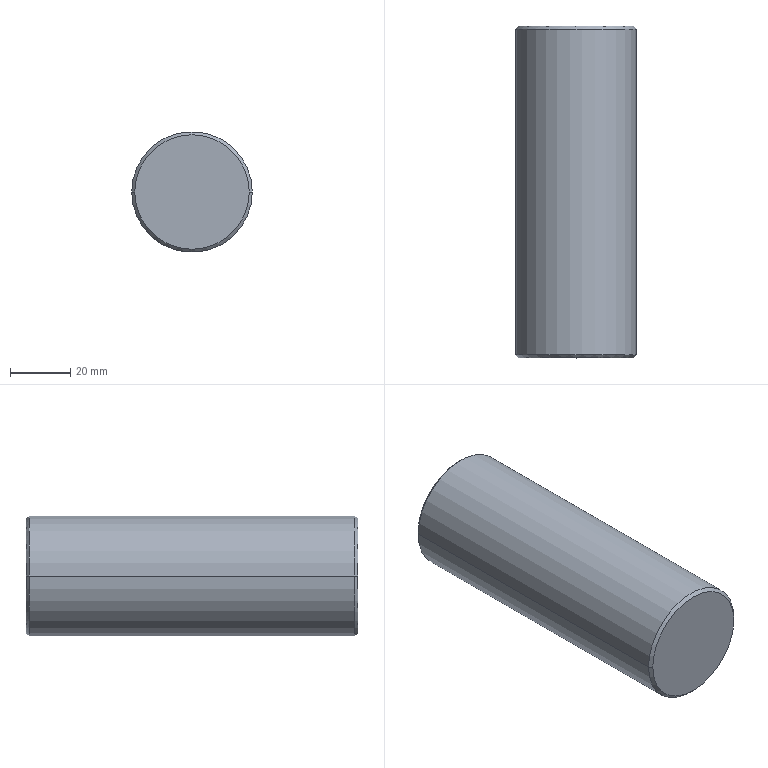Part | SolidWorks | 1 solid | 8 faces | box 40 x 110 x 40 mm | volume 138107 mm3 | cone 4 | cylinder 2 | plane 2 | commonest cylinder face diameters 40 x2
STEP:
#1=CARTESIAN_POINT('',(-19.,0.,0.));
#2=VERTEX_POINT('',#1);
#3=CARTESIAN_POINT('',(19.,0.,0.));
#4=VERTEX_POINT('',#3);
#5=CARTESIAN_POINT('',(0.,0.,0.));
#6=DIRECTION('',(0.,1.,0.));
#7=DIRECTION('',(-1.,0.,0.));
#8=AXIS2_PLACEMENT_3D('',#5,#6,#7);
#9=CIRCLE('',#8,19.);
#10=EDGE_CURVE('',#2,#4,#9,.T.);
#11=ORIENTED_EDGE('',*,*,#10,.F.);
#12=CARTESIAN_POINT('',(-20.,-1.,0.));
#13=VERTEX_POINT('',#12);
#14=CARTESIAN_POINT('',(-20.,-1.,0.));
#15=DIRECTION('',(-0.7071,-0.7071,0.));
#16=VECTOR('',#15,1000.);
#17=LINE('',#14,#16);
#18=EDGE_CURVE('',#2,#13,#17,.T.);
#19=ORIENTED_EDGE('',*,*,#18,.T.);
#20=CARTESIAN_POINT('',(20.,-1.,0.));
#21=VERTEX_POINT('',#20);
#22=CARTESIAN_POINT('',(0.,-1.,0.));
#23=DIRECTION('',(0.,1.,0.));
#24=DIRECTION('',(-1.,0.,0.));
#25=AXIS2_PLACEMENT_3D('',#22,#23,#24);
#26=CIRCLE('',#25,20.);
#27=EDGE_CURVE('',#13,#21,#26,.T.);
#28=ORIENTED_EDGE('',*,*,#27,.T.);
#29=CARTESIAN_POINT('',(20.,-1.,0.));
#30=DIRECTION('',(0.7071,-0.7071,0.));
#31=VECTOR('',#30,1000.);
#32=LINE('',#29,#31);
#33=EDGE_CURVE('',#4,#21,#32,.T.);
#34=ORIENTED_EDGE('',*,*,#33,.F.);
#35=EDGE_LOOP('',(#11,#19,#28,#34));
#36=FACE_OUTER_BOUND('',#35,.T.);
#37=CARTESIAN_POINT('',(0.,-1.,0.));
#38=DIRECTION('',(0.,-1.,0.));
#39=DIRECTION('',(1.,0.,0.));
#40=AXIS2_PLACEMENT_3D('',#37,#38,#39);
#41=CONICAL_SURFACE('',#40,20.,0.7854);
#42=ADVANCED_FACE('',(#36),#41,.T.);
#43=CARTESIAN_POINT('',(-20.,-109.,0.));
#44=VERTEX_POINT('',#43);
#45=CARTESIAN_POINT('',(20.,-109.,0.));
#46=VERTEX_POINT('',#45);
#47=CARTESIAN_POINT('',(0.,-109.,0.));
#48=DIRECTION('',(0.,1.,0.));
#49=DIRECTION('',(-1.,0.,0.));
#50=AXIS2_PLACEMENT_3D('',#47,#48,#49);
#51=CIRCLE('',#50,20.);
#52=EDGE_CURVE('',#44,#46,#51,.T.);
#53=ORIENTED_EDGE('',*,*,#52,.T.);
#54=CARTESIAN_POINT('',(20.,0.,0.));
#55=DIRECTION('',(0.,1.,0.));
#56=VECTOR('',#55,1000.);
#57=LINE('',#54,#56);
#58=EDGE_CURVE('',#46,#21,#57,.T.);
#59=ORIENTED_EDGE('',*,*,#58,.T.);
#60=ORIENTED_EDGE('',*,*,#27,.F.);
#61=CARTESIAN_POINT('',(-20.,0.,0.));
#62=DIRECTION('',(0.,1.,0.));
#63=VECTOR('',#62,1000.);
#64=LINE('',#61,#63);
#65=EDGE_CURVE('',#44,#13,#64,.T.);
#66=ORIENTED_EDGE('',*,*,#65,.F.);
#67=EDGE_LOOP('',(#53,#59,#60,#66));
#68=FACE_OUTER_BOUND('',#67,.T.);
#69=CARTESIAN_POINT('',(0.,0.,0.));
#70=DIRECTION('',(0.,1.,0.));
#71=DIRECTION('',(-1.,0.,0.));
#72=AXIS2_PLACEMENT_3D('',#69,#70,#71);
#73=CYLINDRICAL_SURFACE('',#72,20.);
#74=ADVANCED_FACE('',(#68),#73,.T.);
#75=CARTESIAN_POINT('',(-19.,-110.,0.));
#76=VERTEX_POINT('',#75);
#77=CARTESIAN_POINT('',(19.,-110.,0.));
#78=VERTEX_POINT('',#77);
#79=CARTESIAN_POINT('',(0.,-110.,0.));
#80=DIRECTION('',(0.,1.,0.));
#81=DIRECTION('',(-1.,0.,0.));
#82=AXIS2_PLACEMENT_3D('',#79,#80,#81);
#83=CIRCLE('',#82,19.);
#84=EDGE_CURVE('',#76,#78,#83,.T.);
#85=ORIENTED_EDGE('',*,*,#84,.T.);
#86=CARTESIAN_POINT('',(19.,-110.,0.));
#87=DIRECTION('',(0.7071,0.7071,0.));
#88=VECTOR('',#87,1000.);
#89=LINE('',#86,#88);
#90=EDGE_CURVE('',#78,#46,#89,.T.);
#91=ORIENTED_EDGE('',*,*,#90,.T.);
#92=ORIENTED_EDGE('',*,*,#52,.F.);
#93=CARTESIAN_POINT('',(-19.,-110.,0.));
#94=DIRECTION('',(-0.7071,0.7071,0.));
#95=VECTOR('',#94,1000.);
#96=LINE('',#93,#95);
#97=EDGE_CURVE('',#76,#44,#96,.T.);
#98=ORIENTED_EDGE('',*,*,#97,.F.);
#99=EDGE_LOOP('',(#85,#91,#92,#98));
#100=FACE_OUTER_BOUND('',#99,.T.);
#101=CARTESIAN_POINT('',(0.,-110.,0.));
#102=DIRECTION('',(0.,1.,0.));
#103=DIRECTION('',(-1.,0.,0.));
#104=AXIS2_PLACEMENT_3D('',#101,#102,#103);
#105=CONICAL_SURFACE('',#104,19.,0.7854);
#106=ADVANCED_FACE('',(#100),#105,.T.);
#107=ORIENTED_EDGE('',*,*,#84,.F.);
#108=CARTESIAN_POINT('',(0.,-110.,0.));
#109=DIRECTION('',(0.,1.,0.));
#110=DIRECTION('',(-1.,0.,0.));
#111=AXIS2_PLACEMENT_3D('',#108,#109,#110);
#112=CIRCLE('',#111,19.);
#113=EDGE_CURVE('',#78,#76,#112,.T.);
#114=ORIENTED_EDGE('',*,*,#113,.F.);
#115=EDGE_LOOP('',(#107,#114));
#116=FACE_OUTER_BOUND('',#115,.T.);
#117=CARTESIAN_POINT('',(0.,-110.,0.));
#118=DIRECTION('',(0.,1.,0.));
#119=DIRECTION('',(-1.,0.,0.));
#120=AXIS2_PLACEMENT_3D('',#117,#118,#119);
#121=PLANE('',#120);
#122=ADVANCED_FACE('',(#116),#121,.F.);
#123=ORIENTED_EDGE('',*,*,#90,.F.);
#124=ORIENTED_EDGE('',*,*,#113,.T.);
#125=ORIENTED_EDGE('',*,*,#97,.T.);
#126=CARTESIAN_POINT('',(0.,-109.,0.));
#127=DIRECTION('',(0.,1.,0.));
#128=DIRECTION('',(-1.,0.,0.));
#129=AXIS2_PLACEMENT_3D('',#126,#127,#128);
#130=CIRCLE('',#129,20.);
#131=EDGE_CURVE('',#46,#44,#130,.T.);
#132=ORIENTED_EDGE('',*,*,#131,.F.);
#133=EDGE_LOOP('',(#123,#124,#125,#132));
#134=FACE_OUTER_BOUND('',#133,.T.);
#135=CARTESIAN_POINT('',(0.,-110.,0.));
#136=DIRECTION('',(0.,1.,0.));
#137=DIRECTION('',(-1.,0.,0.));
#138=AXIS2_PLACEMENT_3D('',#135,#136,#137);
#139=CONICAL_SURFACE('',#138,19.,0.7854);
#140=ADVANCED_FACE('',(#134),#139,.T.);
#141=ORIENTED_EDGE('',*,*,#58,.F.);
#142=ORIENTED_EDGE('',*,*,#131,.T.);
#143=ORIENTED_EDGE('',*,*,#65,.T.);
#144=CARTESIAN_POINT('',(0.,-1.,0.));
#145=DIRECTION('',(0.,1.,0.));
#146=DIRECTION('',(-1.,0.,0.));
#147=AXIS2_PLACEMENT_3D('',#144,#145,#146);
#148=CIRCLE('',#147,20.);
#149=EDGE_CURVE('',#21,#13,#148,.T.);
#150=ORIENTED_EDGE('',*,*,#149,.F.);
#151=EDGE_LOOP('',(#141,#142,#143,#150));
#152=FACE_OUTER_BOUND('',#151,.T.);
#153=CARTESIAN_POINT('',(0.,0.,0.));
#154=DIRECTION('',(0.,1.,0.));
#155=DIRECTION('',(-1.,0.,0.));
#156=AXIS2_PLACEMENT_3D('',#153,#154,#155);
#157=CYLINDRICAL_SURFACE('',#156,20.);
#158=ADVANCED_FACE('',(#152),#157,.T.);
#159=ORIENTED_EDGE('',*,*,#18,.F.);
#160=CARTESIAN_POINT('',(0.,0.,0.));
#161=DIRECTION('',(0.,1.,0.));
#162=DIRECTION('',(-1.,0.,0.));
#163=AXIS2_PLACEMENT_3D('',#160,#161,#162);
#164=CIRCLE('',#163,19.);
#165=EDGE_CURVE('',#4,#2,#164,.T.);
#166=ORIENTED_EDGE('',*,*,#165,.F.);
#167=ORIENTED_EDGE('',*,*,#33,.T.);
#168=ORIENTED_EDGE('',*,*,#149,.T.);
#169=EDGE_LOOP('',(#159,#166,#167,#168));
#170=FACE_OUTER_BOUND('',#169,.T.);
#171=CARTESIAN_POINT('',(0.,-1.,0.));
#172=DIRECTION('',(0.,-1.,0.));
#173=DIRECTION('',(1.,0.,0.));
#174=AXIS2_PLACEMENT_3D('',#171,#172,#173);
#175=CONICAL_SURFACE('',#174,20.,0.7854);
#176=ADVANCED_FACE('',(#170),#175,.T.);
#177=ORIENTED_EDGE('',*,*,#165,.T.);
#178=ORIENTED_EDGE('',*,*,#10,.T.);
#179=EDGE_LOOP('',(#177,#178));
#180=FACE_OUTER_BOUND('',#179,.T.);
#181=CARTESIAN_POINT('',(0.,0.,0.));
#182=DIRECTION('',(0.,-1.,0.));
#183=DIRECTION('',(1.,0.,0.));
#184=AXIS2_PLACEMENT_3D('',#181,#182,#183);
#185=PLANE('',#184);
#186=ADVANCED_FACE('',(#180),#185,.F.);
#187=CLOSED_SHELL('',(#42,#74,#106,#122,#140,#158,#176,#186));
#188=MANIFOLD_SOLID_BREP('',#187);
#189=CARTESIAN_POINT('',(0.,0.,0.));
#190=DIRECTION('',(0.,0.,1.));
#191=DIRECTION('',(1.,0.,0.));
#192=AXIS2_PLACEMENT_3D('',#189,#190,#191);
#193=(LENGTH_UNIT()NAMED_UNIT(*)SI_UNIT(.MILLI.,.METRE.));
#194=UNCERTAINTY_MEASURE_WITH_UNIT(LENGTH_MEASURE(0.00001),#193,'','');
#195=(NAMED_UNIT(*)PLANE_ANGLE_UNIT()SI_UNIT($,.RADIAN.));
#196=(NAMED_UNIT(*)SI_UNIT($,.STERADIAN.)SOLID_ANGLE_UNIT());
#197=(GEOMETRIC_REPRESENTATION_CONTEXT(3)GLOBAL_UNCERTAINTY_ASSIGNED_CONTEXT((#194))GLOBAL_UNIT_ASSIGNED_CONTEXT((#193,#195,#196))REPRESENTATION_CONTEXT('',''));
#198=ADVANCED_BREP_SHAPE_REPRESENTATION('',(#188,#192),#197);